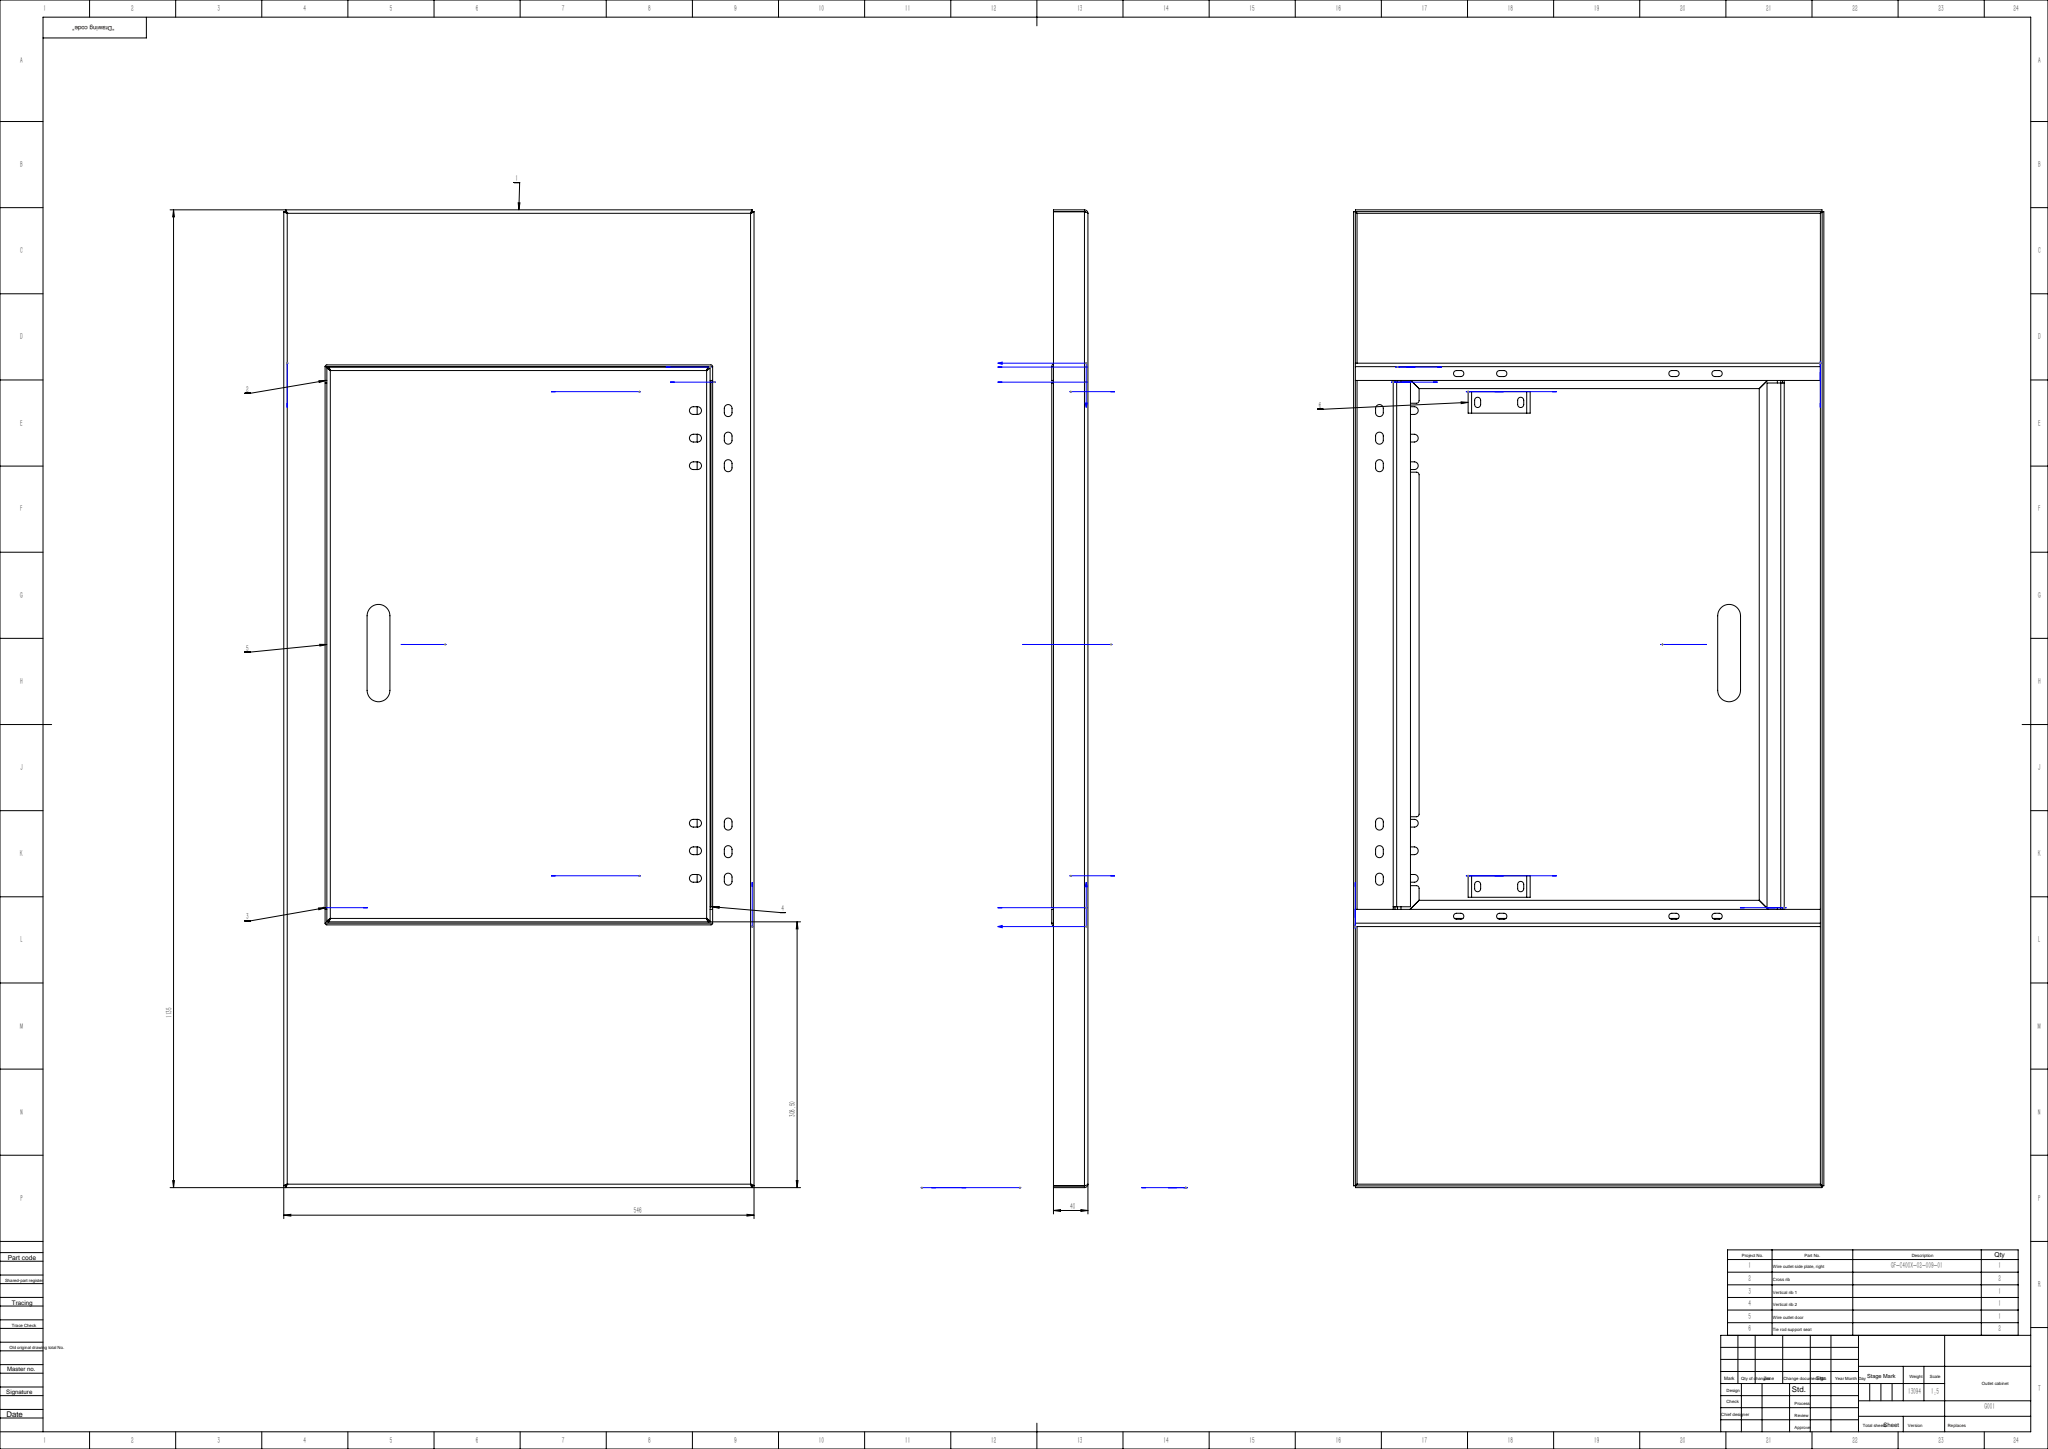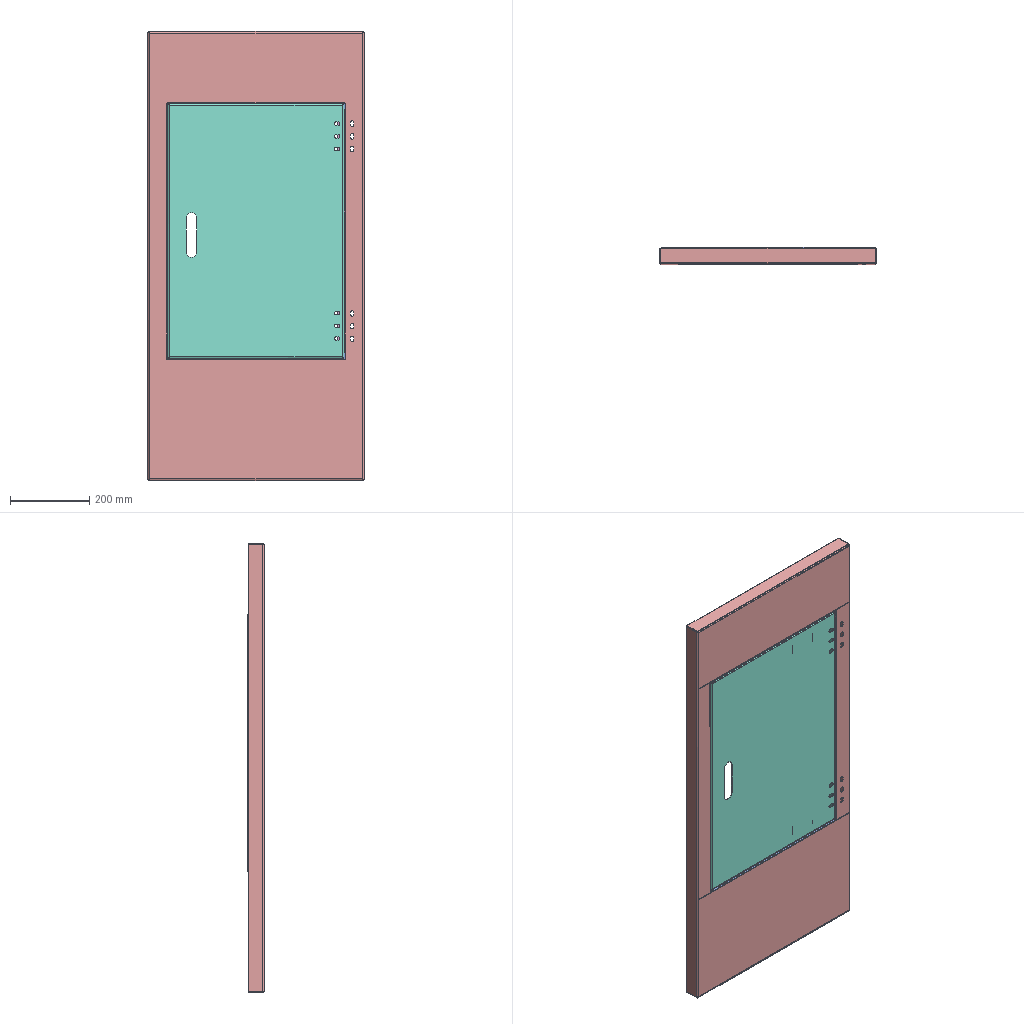Assembly | SolidWorks | 9 different items | 11 placed | box 546 x 42 x 1135 mm
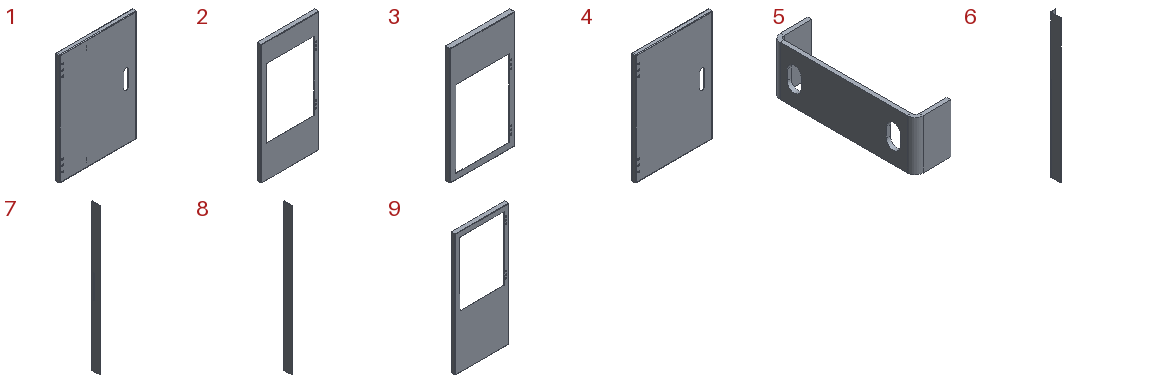Parts list (item | name | quantity | parent item | size | volume | features):
1 | (subassembly) | x1 | - | 445 x 25 x 644 mm | 754672 mm3 | -
2 | - | x1 | - | 546 x 40 x 1135 mm | 898640 mm3 | features ICE 2, EdgeFlange 1, FlatPattern 1, SMBaseFlange 1, SheetMetal 1
3 | - | x1 | - | 546 x 40 x 985 mm | 712813 mm3 | features ICE 2, EdgeFlange 1, FlatPattern 1, SMBaseFlange 1, SheetMetal 1
4 | - | x1 | in 1 | 445 x 25 x 644 mm | 745118 mm3 | features CornerFeat 4, ICE 3, EdgeFlange 2, Fillet 1, FlatPattern 1, SMBaseFlange 1, SheetMetal 1
5 | - | x2 | in 1 | 18 x 72 x 25 mm | 4777 mm3 | features FlatPattern 1, ICE 1, SMBaseFlange 1, SheetMetal 1
6 | - | x2 | - | 20 x 40 x 540 mm | 60662 mm3 | features FlatPattern 1, ICE 1, SMBaseFlange 1, SheetMetal 1
7 | - | x1 | - | 20 x 40 x 649 mm | 70699 mm3 | features SMBaseFlange 2, FlatPattern 1, ICE 1, SheetMetal 1
8 | - | x1 | - | 20 x 40 x 649 mm | 71956 mm3 | features SMBaseFlange 2, FlatPattern 1, SheetMetal 1
9 | - | x1 | - | 546 x 40 x 1245 mm | 1034914 mm3 | features ICE 2, EdgeFlange 1, FlatPattern 1, SMBaseFlange 1, SheetMetal 1
Mates (type | each side: item.copy, entity, surface, feature):
In the top assembly
Coincident | 2.1 face plane Base-Flange1 | 6.1 face plane Base-Flange1
Coincident | 2.1 face plane Edge-Flange1 | 6.1 face plane Base-Flange1
Coincident | 2.1 face plane Cut-Extrude1 | 6.1 face plane Base-Flange1
Coincident | 2.1 face plane Edge-Flange1 | 6.2 face plane Base-Flange1
Coincident | 2.1 face plane Base-Flange1 | 6.2 face plane Base-Flange1
Coincident | 2.1 face plane Cut-Extrude1 | 6.2 face plane Base-Flange1
Coincident | 2.1 face plane Base-Flange1 | 7.1 face plane Base-Flange1
Coincident | 6.2 face plane Base-Flange1 | 7.1 face plane Thin sheet 1
Coincident | 2.1 face plane Cut-Extrude1 | 7.1 face plane Base-Flange1
Coincident | 6.1 face plane Base-Flange1 | 8.1 face plane Thin sheet 1
Coincident | 2.1 face plane Base-Flange1 | 8.1 face plane Base-Flange1
Coincident | 2.1 face plane Cut-Extrude1 | 8.1 face plane Base-Flange1
Coincident | 2.1 face plane Base-Flange1 | 4.1 face plane Base-Flange1
DistanceDim | 4.1 face plane Edge-Flange1 | 6.1 face plane Base-Flange1
DistanceDim | 4.1 face plane Edge-Flange1 | 2.1 face plane Cut-Extrude1
In subassembly 1
Coincident | 4.2 face plane Base-Flange1 | 5.1 face plane Base-Flange1
DistanceDim | 5.1 face plane Base-Flange1 | 4.2 face plane Edge-Flange1 | 2 times
Coincident | 4.2 face plane Base-Flange1 | 5.2 face plane Base-Flange1
DistanceDim | 5.2 face plane Base-Flange1 | 4.2 face plane Edge-Flange1
DistanceDim | 4.2 face plane Edge-Flange1 | 5.2 face plane Base-Flange1